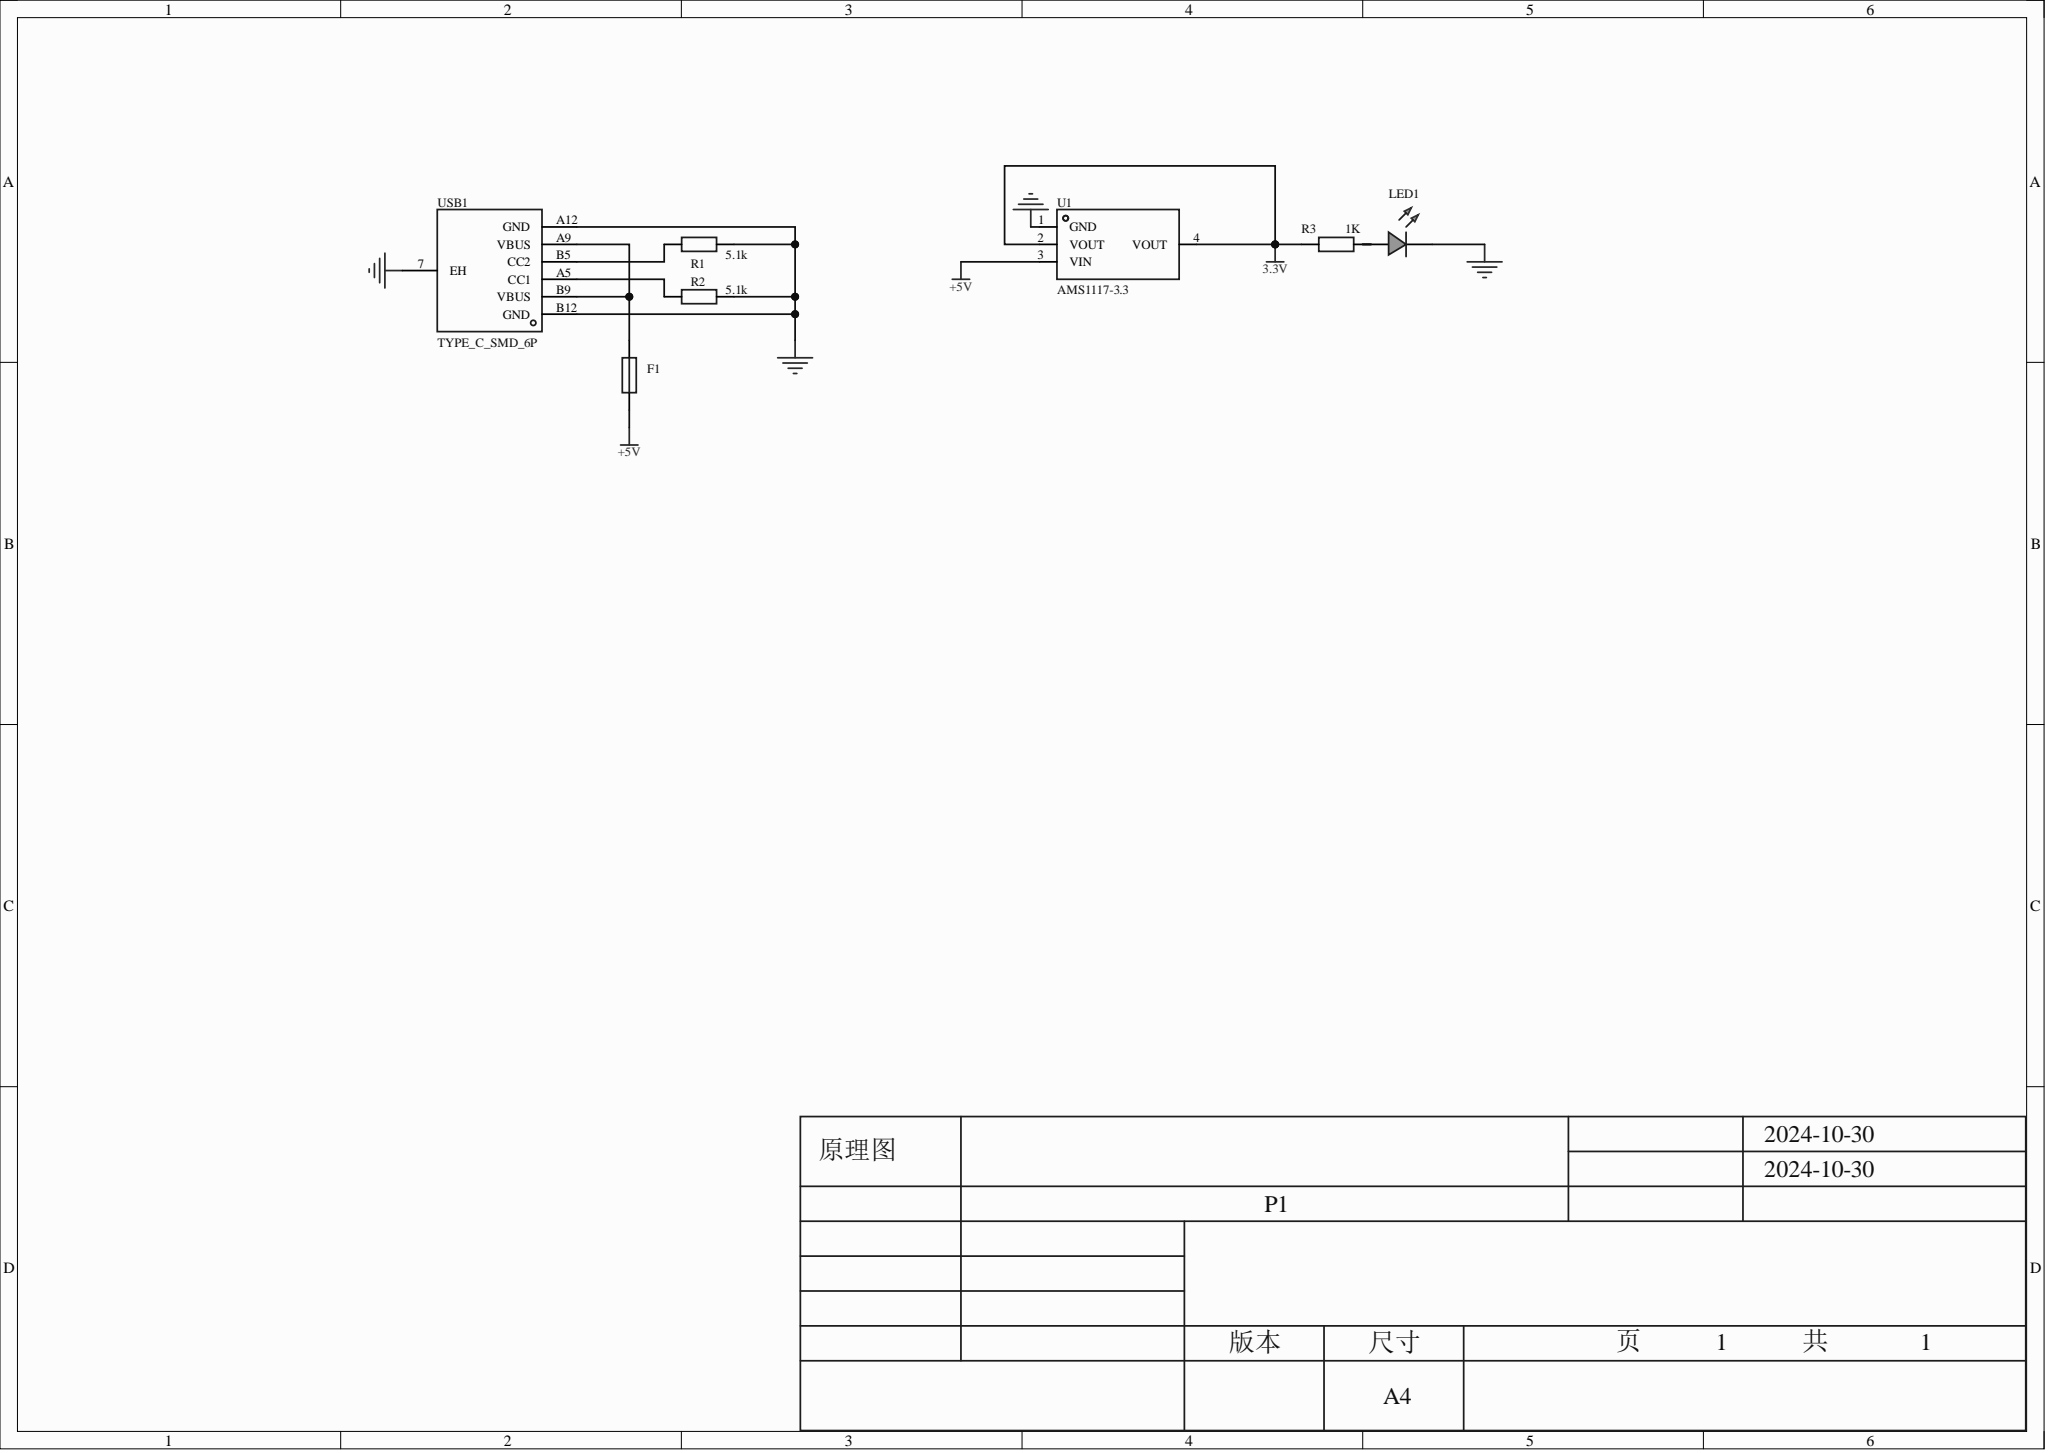Circuit board | Altium Designer | 7 parts | 7 nets
Bill of materials:
Comment,Description,Designator,Footprint,LibRef,Quantity
"BSMD1206-200-6V","","F1","F1206","BSMD1206-200-6V","1"
"","","LED1","LED_0805","LED_0805-G","1"
"5.1k","","R1, R2","R0805","Res_0805","2"
"1K","","R3","R0603","Res_0603","1"
"AMS1117-3.3","","U1","SOT-223-3_L6.5-W3.4-P2.30-LS7.0-BR","AMS1117-3.3_C6186","1"
"TYPE_C_SMD_6P","","USB1","TYPE-C-SMD_TYPE-C-6P","TYPE_C_SMD_6P","1"
Netlist (Protel format):
[
F1
F1206
BSMD1206-200-6V



]
[
LED1
LED_0805




]
[
R1
R0805
5.1k



]
[
R2
R0805
5.1k



]
[
R3
R0603
1K



]
[
U1
SOT-223-3_L6.5-W3.4-P2.30-LS7.0-BR
AMS1117-3.3



]
[
USB1
TYPE-C-SMD_TYPE-C-6P
TYPE_C_SMD_6P



]
(
NetR2_1
R2-1
USB1-A5
)
(
NetR1_1
R1-1
USB1-B5
)
(
NetLED1_2
LED1-2
R3-2
)
(
NetF1_2
F1-2
USB1-A9
USB1-B9
)
(
GND
LED1-1
R1-2
R2-2
U1-1
USB1-7
USB1-A12
USB1-B12
)
(
+5V
F1-1
U1-3
)
(
3.3V
R3-1
U1-2
U1-4
)